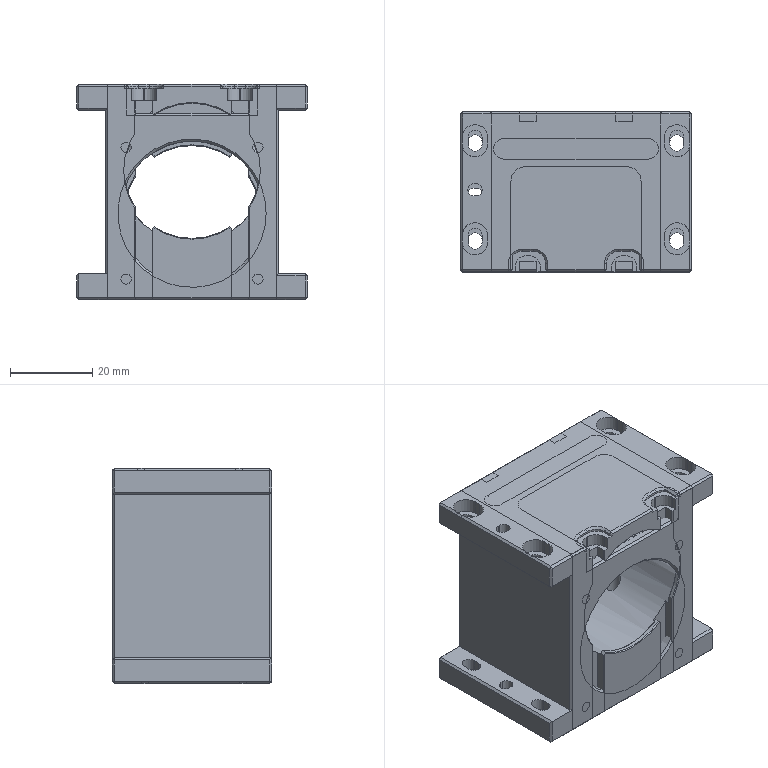NC program | NX | posted with a generic post | part box 56 x 38.8 x 52.3 mm
Lines 1 to 18 of 18366:
N10 G17 G21 G94 G90
(飞顶面D50 , TOOL : 飞刀D50)
N12 T20 M6
N14 G54
N16 G17 G0 G90 X58. Y0. S5500 M3
N18 G43 Z33. H20
N20 Z2.
N22 G94 G1 Z0. F1200.
N24 X53.
N26 X-53.
N28 X-58.
N30 Z2.
N32 G0 Z33.
N34 M5